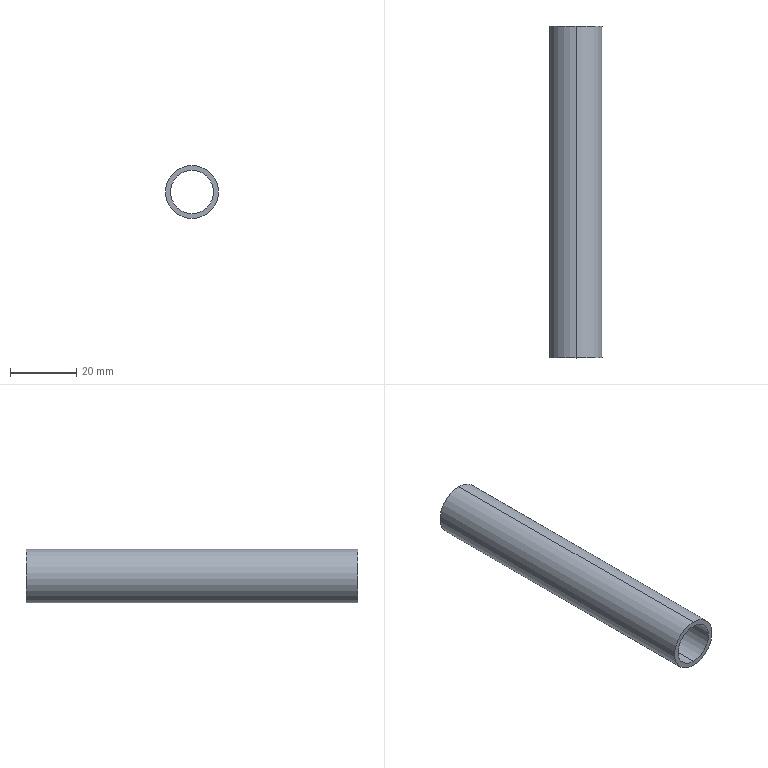Part | SolidWorks | features Sweep 1 | 1 solid | 6 faces | box 16 x 100 x 16 mm | volume 6833 mm3 | cylinder 4 | plane 2 | commonest cylinder face diameters 13 x2 16 x2
STEP:
#1=CARTESIAN_POINT('',(0.,0.,-6.5));
#2=VERTEX_POINT('',#1);
#3=CARTESIAN_POINT('',(0.,0.,6.5));
#4=VERTEX_POINT('',#3);
#5=CARTESIAN_POINT('',(0.,0.,0.));
#6=DIRECTION('',(0.,1.,0.));
#7=DIRECTION('',(0.,0.,1.));
#8=AXIS2_PLACEMENT_3D('',#5,#6,#7);
#9=CIRCLE('',#8,6.5);
#10=EDGE_CURVE('',#2,#4,#9,.T.);
#11=ORIENTED_EDGE('',*,*,#10,.F.);
#12=CARTESIAN_POINT('',(0.,100.,-6.5));
#13=VERTEX_POINT('',#12);
#14=CARTESIAN_POINT('',(0.,0.,-6.5));
#15=DIRECTION('',(0.,1.,0.));
#16=VECTOR('',#15,1000.);
#17=LINE('',#14,#16);
#18=EDGE_CURVE('',#2,#13,#17,.T.);
#19=ORIENTED_EDGE('',*,*,#18,.T.);
#20=CARTESIAN_POINT('',(0.,100.,6.5));
#21=VERTEX_POINT('',#20);
#22=CARTESIAN_POINT('',(0.,100.,0.));
#23=DIRECTION('',(0.,1.,0.));
#24=DIRECTION('',(0.,0.,1.));
#25=AXIS2_PLACEMENT_3D('',#22,#23,#24);
#26=CIRCLE('',#25,6.5);
#27=EDGE_CURVE('',#13,#21,#26,.T.);
#28=ORIENTED_EDGE('',*,*,#27,.T.);
#29=CARTESIAN_POINT('',(0.,0.,6.5));
#30=DIRECTION('',(0.,1.,0.));
#31=VECTOR('',#30,1000.);
#32=LINE('',#29,#31);
#33=EDGE_CURVE('',#4,#21,#32,.T.);
#34=ORIENTED_EDGE('',*,*,#33,.F.);
#35=EDGE_LOOP('',(#11,#19,#28,#34));
#36=FACE_OUTER_BOUND('',#35,.T.);
#37=CARTESIAN_POINT('',(0.,0.,0.));
#38=DIRECTION('',(0.,1.,0.));
#39=DIRECTION('',(0.,0.,1.));
#40=AXIS2_PLACEMENT_3D('',#37,#38,#39);
#41=CYLINDRICAL_SURFACE('',#40,6.5);
#42=ADVANCED_FACE('',(#36),#41,.F.);
#43=CARTESIAN_POINT('',(0.,0.,8.));
#44=VERTEX_POINT('',#43);
#45=CARTESIAN_POINT('',(0.,0.,-8.));
#46=VERTEX_POINT('',#45);
#47=CARTESIAN_POINT('',(0.,0.,0.));
#48=DIRECTION('',(0.,1.,0.));
#49=DIRECTION('',(0.,0.,1.));
#50=AXIS2_PLACEMENT_3D('',#47,#48,#49);
#51=CIRCLE('',#50,8.);
#52=EDGE_CURVE('',#44,#46,#51,.T.);
#53=ORIENTED_EDGE('',*,*,#52,.T.);
#54=CARTESIAN_POINT('',(0.,100.,-8.));
#55=VERTEX_POINT('',#54);
#56=CARTESIAN_POINT('',(0.,0.,-8.));
#57=DIRECTION('',(0.,1.,0.));
#58=VECTOR('',#57,1000.);
#59=LINE('',#56,#58);
#60=EDGE_CURVE('',#46,#55,#59,.T.);
#61=ORIENTED_EDGE('',*,*,#60,.T.);
#62=CARTESIAN_POINT('',(0.,100.,8.));
#63=VERTEX_POINT('',#62);
#64=CARTESIAN_POINT('',(0.,100.,0.));
#65=DIRECTION('',(0.,1.,0.));
#66=DIRECTION('',(0.,0.,1.));
#67=AXIS2_PLACEMENT_3D('',#64,#65,#66);
#68=CIRCLE('',#67,8.);
#69=EDGE_CURVE('',#63,#55,#68,.T.);
#70=ORIENTED_EDGE('',*,*,#69,.F.);
#71=CARTESIAN_POINT('',(0.,0.,8.));
#72=DIRECTION('',(0.,1.,0.));
#73=VECTOR('',#72,1000.);
#74=LINE('',#71,#73);
#75=EDGE_CURVE('',#44,#63,#74,.T.);
#76=ORIENTED_EDGE('',*,*,#75,.F.);
#77=EDGE_LOOP('',(#53,#61,#70,#76));
#78=FACE_OUTER_BOUND('',#77,.T.);
#79=CARTESIAN_POINT('',(0.,0.,0.));
#80=DIRECTION('',(0.,1.,0.));
#81=DIRECTION('',(0.,0.,1.));
#82=AXIS2_PLACEMENT_3D('',#79,#80,#81);
#83=CYLINDRICAL_SURFACE('',#82,8.);
#84=ADVANCED_FACE('',(#78),#83,.T.);
#85=ORIENTED_EDGE('',*,*,#60,.F.);
#86=CARTESIAN_POINT('',(0.,0.,0.));
#87=DIRECTION('',(0.,1.,0.));
#88=DIRECTION('',(0.,0.,1.));
#89=AXIS2_PLACEMENT_3D('',#86,#87,#88);
#90=CIRCLE('',#89,8.);
#91=EDGE_CURVE('',#46,#44,#90,.T.);
#92=ORIENTED_EDGE('',*,*,#91,.T.);
#93=ORIENTED_EDGE('',*,*,#75,.T.);
#94=CARTESIAN_POINT('',(0.,100.,0.));
#95=DIRECTION('',(0.,1.,0.));
#96=DIRECTION('',(0.,0.,1.));
#97=AXIS2_PLACEMENT_3D('',#94,#95,#96);
#98=CIRCLE('',#97,8.);
#99=EDGE_CURVE('',#55,#63,#98,.T.);
#100=ORIENTED_EDGE('',*,*,#99,.F.);
#101=EDGE_LOOP('',(#85,#92,#93,#100));
#102=FACE_OUTER_BOUND('',#101,.T.);
#103=CARTESIAN_POINT('',(0.,0.,0.));
#104=DIRECTION('',(0.,1.,0.));
#105=DIRECTION('',(0.,0.,1.));
#106=AXIS2_PLACEMENT_3D('',#103,#104,#105);
#107=CYLINDRICAL_SURFACE('',#106,8.);
#108=ADVANCED_FACE('',(#102),#107,.T.);
#109=CARTESIAN_POINT('',(0.,100.,0.));
#110=DIRECTION('',(0.,1.,0.));
#111=DIRECTION('',(0.,0.,1.));
#112=AXIS2_PLACEMENT_3D('',#109,#110,#111);
#113=CIRCLE('',#112,6.5);
#114=EDGE_CURVE('',#21,#13,#113,.T.);
#115=ORIENTED_EDGE('',*,*,#114,.F.);
#116=ORIENTED_EDGE('',*,*,#27,.F.);
#117=EDGE_LOOP('',(#115,#116));
#118=FACE_BOUND('',#117,.T.);
#119=ORIENTED_EDGE('',*,*,#69,.T.);
#120=ORIENTED_EDGE('',*,*,#99,.T.);
#121=EDGE_LOOP('',(#119,#120));
#122=FACE_OUTER_BOUND('',#121,.T.);
#123=CARTESIAN_POINT('',(0.,100.,0.));
#124=DIRECTION('',(0.,1.,0.));
#125=DIRECTION('',(0.,0.,1.));
#126=AXIS2_PLACEMENT_3D('',#123,#124,#125);
#127=PLANE('',#126);
#128=ADVANCED_FACE('',(#118,#122),#127,.T.);
#129=CARTESIAN_POINT('',(0.,0.,0.));
#130=DIRECTION('',(0.,1.,0.));
#131=DIRECTION('',(0.,0.,1.));
#132=AXIS2_PLACEMENT_3D('',#129,#130,#131);
#133=CIRCLE('',#132,6.5);
#134=EDGE_CURVE('',#4,#2,#133,.T.);
#135=ORIENTED_EDGE('',*,*,#134,.T.);
#136=ORIENTED_EDGE('',*,*,#10,.T.);
#137=EDGE_LOOP('',(#135,#136));
#138=FACE_BOUND('',#137,.T.);
#139=ORIENTED_EDGE('',*,*,#52,.F.);
#140=ORIENTED_EDGE('',*,*,#91,.F.);
#141=EDGE_LOOP('',(#139,#140));
#142=FACE_OUTER_BOUND('',#141,.T.);
#143=CARTESIAN_POINT('',(0.,0.,0.));
#144=DIRECTION('',(0.,1.,0.));
#145=DIRECTION('',(0.,0.,1.));
#146=AXIS2_PLACEMENT_3D('',#143,#144,#145);
#147=PLANE('',#146);
#148=ADVANCED_FACE('',(#138,#142),#147,.F.);
#149=ORIENTED_EDGE('',*,*,#18,.F.);
#150=ORIENTED_EDGE('',*,*,#134,.F.);
#151=ORIENTED_EDGE('',*,*,#33,.T.);
#152=ORIENTED_EDGE('',*,*,#114,.T.);
#153=EDGE_LOOP('',(#149,#150,#151,#152));
#154=FACE_OUTER_BOUND('',#153,.T.);
#155=CARTESIAN_POINT('',(0.,0.,0.));
#156=DIRECTION('',(0.,1.,0.));
#157=DIRECTION('',(0.,0.,1.));
#158=AXIS2_PLACEMENT_3D('',#155,#156,#157);
#159=CYLINDRICAL_SURFACE('',#158,6.5);
#160=ADVANCED_FACE('',(#154),#159,.F.);
#161=CLOSED_SHELL('',(#42,#84,#108,#128,#148,#160));
#162=MANIFOLD_SOLID_BREP('',#161);
#163=CARTESIAN_POINT('',(0.,0.,0.));
#164=DIRECTION('',(0.,0.,1.));
#165=DIRECTION('',(1.,0.,0.));
#166=AXIS2_PLACEMENT_3D('',#163,#164,#165);
#167=(LENGTH_UNIT()NAMED_UNIT(*)SI_UNIT(.MILLI.,.METRE.));
#168=UNCERTAINTY_MEASURE_WITH_UNIT(LENGTH_MEASURE(0.00001),#167,'','');
#169=(NAMED_UNIT(*)PLANE_ANGLE_UNIT()SI_UNIT($,.RADIAN.));
#170=(NAMED_UNIT(*)SI_UNIT($,.STERADIAN.)SOLID_ANGLE_UNIT());
#171=(GEOMETRIC_REPRESENTATION_CONTEXT(3)GLOBAL_UNCERTAINTY_ASSIGNED_CONTEXT((#168))GLOBAL_UNIT_ASSIGNED_CONTEXT((#167,#169,#170))REPRESENTATION_CONTEXT('',''));
#172=ADVANCED_BREP_SHAPE_REPRESENTATION('',(#162,#166),#171);